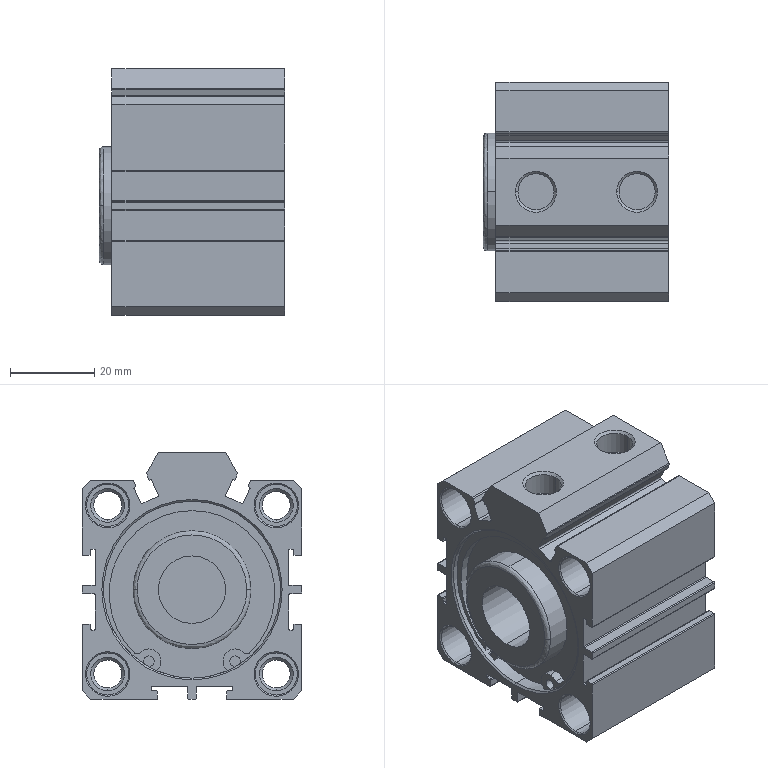Part | STEP file | 1_11 | 1 solid | 230 faces | box 44 x 52 x 58.5 mm | volume 61531 mm3 | cylinder 106 | plane 82 | cone 40 | spline 2 | commonest cylinder face diameters 0.4 x46 10 x16 0.8 x8 6.647 x8 2.5 x6 5.8 x4